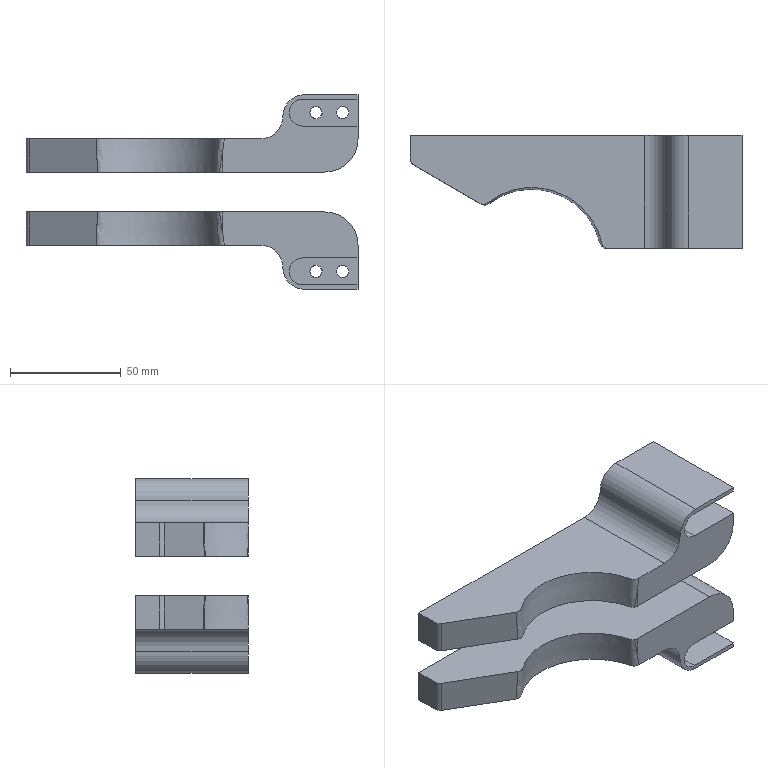NC program | NX | posted with a generic post | part box 150 x 51 x 88 mm
Lines 1 to 42 of 21230:
N10 G17 G21 G94 G90
(FLOOR_WALL_COPY , TOOL : D63)
N12 T01 M6
N14 G54
N16 G17 G0 G90 X112.499 Y0. S6500 M3
N18 G43 Z30. H1
N20 Z3.
N22 G94 G1 Z0. F1500.
N24 X109.499
N26 X-109.5
N28 X-112.5
N30 Z3.
N32 G0 Z30.
N34 M5
(DRILLING_COPY_1 , TOOL : D6A45)
N36 T07 M6
N38 G54
N40 G17 G0 G90 X56. Y-9.4 S5000 M3
N42 G43 Z30. H7
N44 G94 G81 G98 Z-1. F250. R3.
N46 X68.
N48 G80
N50 G0 X68. Y-9.4 Z30.
N52 M5
(DRILLING_COPY_COPY , TOOL : 5.5ZT)
N54 T15 M6
N56 G54
N58 G17 G0 G90 X56. Y-9.4 S2000 M3
N60 G43 Z30. H15
N62 G94 G83 G98 Z-53.652 F120. Q2. R3.
N64 X68.
N66 G80
N68 G0 X68. Y-9.4 Z30.
N70 M5